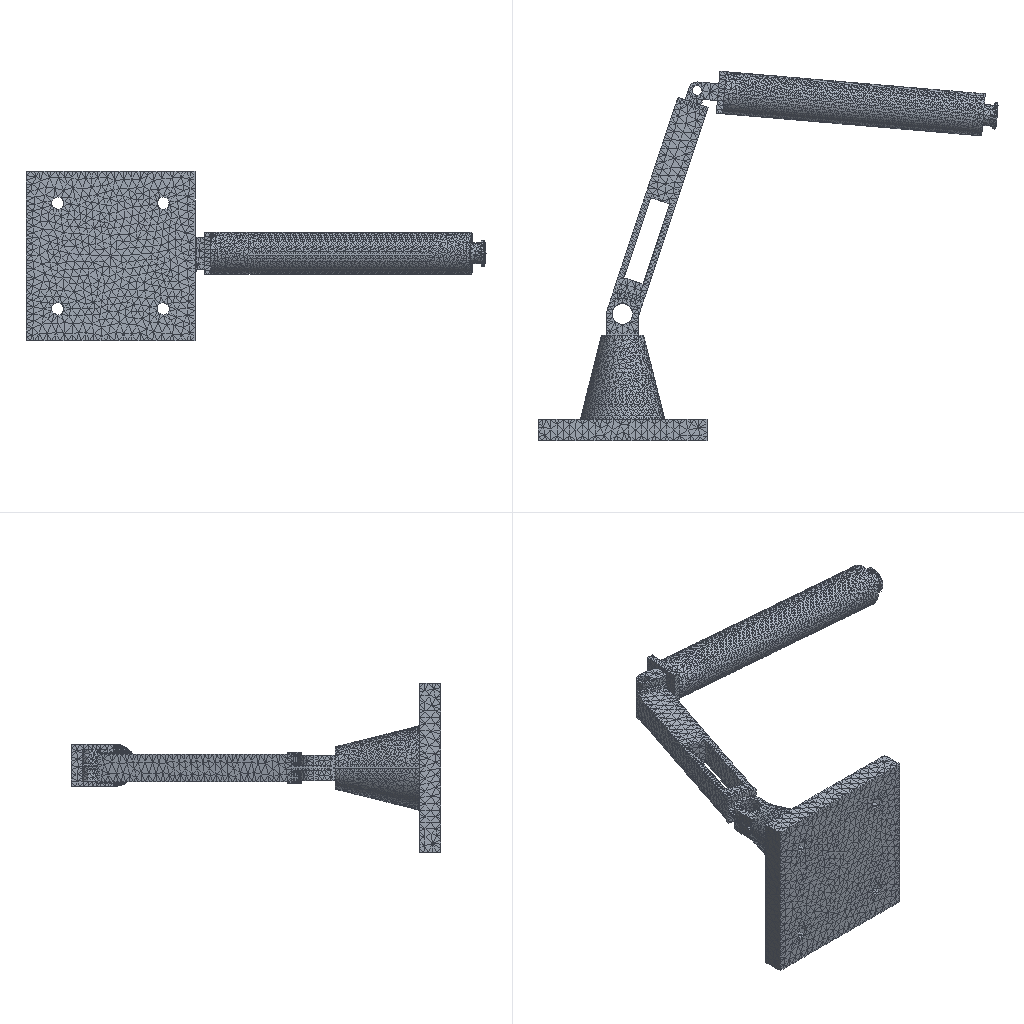Simulation study | ansys workbench
Set-up summary:
category,name,step,type,value,unit,region
solver,ansys_mapdl
solver,version,,,21.1
units,MPA,,stated
analysis,deck,,static,static
load_step,requested,,,1
analysis,nlgeom,,,False
mesh,nodes,,,56505
mesh,elements,,,31911
element_type,ANSYS 187 (type 1),,solid,13480
element_type,ANSYS 187 (type 2),,solid,17937
element_type,ANSYS 174 (type 3),,contact,228
element_type,ANSYS 170 (type 4),,target,228
element_type,ANSYS 154 (type 5),,surface,38
load,load commands in deck,,count,3
bc,support commands in deck,,count,2
named_set,_FIXEDSU,,component
named_set,_FRICSUY,,component
material,1,,in results
material,2,,in results
check,setup vs results,,match,38 surface effect element(s) are not in the reader's mesh and were not compared
Ansys APDL input file, long lists of numbers shortened:
/batch
/config,noeldb,1     ! force off writing results to database
*get,_wallstrt,active,,time,wall
! ANSYS input file written by Workbench version 2021 R1
! File used for geometry attach: D:\仿真\2026.07.04作业分析\模型0706\装配体0706.STEP
/title,____--____ (C5)
! ****** Begin Custom Load Command Snippet ******
/COM, ACT Extensions:
/COM,     LSDYNA, 2021.1
/COM,
! ****** End   Custom Load Command Snippet ******
*DIM,_wb_ProjectScratch_dir,string,248
_wb_ProjectScratch_dir(1) = 'D:\仿真\2026.07.04作业分析\_ProjectScratch\Scr1F88\'
*DIM,_wb_SolverFiles_dir,string,248
_wb_SolverFiles_dir(1) = 'D:\仿真\2026.07.04作业分析\作业分析_files\dp0\SYS-2\MECH\'
*DIM,_wb_userfiles_dir,string,248
_wb_userfiles_dir(1) = 'D:\仿真\2026.07.04作业分析\作业分析_files\user_files\'
/com,--- Data in consistent NMM units. See Solving Units in the help system for more information.
/units,MPA
/nopr
/wb,file,start              !  signify a WB generated input file
/prep7
! Turn off shape checking because checks already performed inside WB mesher.
! See help system for more information.
SHPP,OFF,,NOWARN
/nolist
etcon,set             ! allow ANSYS to choose best KEYOP's for 180x elements, resets any applicable keyopt to MAPDL defaults
/com,*********** Nodes for the whole assembly ***********
nblock,3,,62155
(1i9,3e20.9e3)
        1     2.500000000E+02     6.500000000E+01    -3.005750000E+02
! (56504 more lines like these left out)
-1
/wb,elem,start            !  set before creation of elements
/com,*********** Elements for Body 1 "___0706-FreeParts|NONE" ***********
et,1,187
eblock,19,solid,,13480
(19i9)
        1        1        1        1        0        0        0        0       10        0        1     3000     3829     3017     3722    20851    20955    20841    20850
! (26959 more lines like these left out)
-1
/com,*********** Elements for Body 2 "___0706-FreeParts|NONE[2]" ***********
et,2,187
eblock,19,solid,,17937
(19i9)
        2        2        2        2        0        0        0        0       10        0    13481    25671    29248    25799    28703    38830    39536    38828    38829
! (35873 more lines like these left out)
-1
/wb,elem,end               !  done creating elements
/com,*********** Send User Defined Coordinate System(s) ***********
csys,0
toffst,273.15,  ! Temperature offset from absolute zero
/com,*********** Set Reference Temperature ***********
tref,22.
/wb,mat,start              !  starting to send materials
/com,*********** Send Materials ***********
Temperature = 'TEMP' ! Temperature
MP,DENS,1,7.85e-09,	! tonne mm^-3
MP,ALPX,1,1.2e-05,	! C^-1
MP,C,1,434000000,	! mm^2 s^-2 C^-1
MP,KXX,1,60.5,	! tonne mm s^-3 C^-1
MP,RSVX,1,0.00017,	! ohm mm
MP,EX,1,200000,	! tonne s^-2 mm^-1
MP,NUXY,1,0.3,
MP,MURX,1,10000,
Temperature = 'TEMP' ! Temperature
MP,DENS,2,2.713e-09,	! tonne mm^-3
MP,EX,2,69040,	! tonne s^-2 mm^-1
MP,NUXY,2,0.33,
MP,ALPX,2,2.278e-05,	! C^-1
MP,KXX,2,155.3,	! tonne mm s^-3 C^-1
MP,C,2,915700000,	! mm^2 s^-2 C^-1
/wb,mat,end                !  done sending materials
!************************* Model Summary ********************
!___0706-FreeParts|NONE,	结构钢,	matid,	1
!___0706-FreeParts|NONE[2],	铝合金，锻造，6061，T6,	matid,	2
!************************* End Model Summary ********************
! get the diagonal of the bounding box. Needed later for other things
*get,_xmin,node,,mnloc,x
*get,_ymin,node,,mnloc,y
*get,_zmin,node,,mnloc,z
*get,_xmax,node,,mxloc,x
*get,_ymax,node,,mxloc,y
*get,_zmax,node,,mxloc,z
_ASMDIAG=(_xmax-_xmin)*(_xmax-_xmin)+(_ymax-_ymin)*(_ymax-_ymin)+(_zmax-_zmin)*(_zmax-_zmin)
_ASMDIAG=SQRT(_ASMDIAG)
/wb,contact,start          !  starting to send contact
/com,*********** Create Contact "接触区域" ***********
/com,            Real Constant Set For Above Contact Is 4 & 3
*set,tid,4
*set,cid,3
r,tid
r,cid
et,tid,170
et,cid,174
eblock,10,,,104
(15i9)
    45146        4        4        4        0      156      866      867      867     4869     8828      867     4870
! (103 more lines like these left out)
-1
eblock,10,,,104
(15i9)
    45250        3        3        3        0      156      866      867      867     4869     8828      867     4870
! (103 more lines like these left out)
-1
eblock,10,,,124
(15i9)
    45354        3        4        3        0    24038    24402    24401    24401    29673    31552    24401    29672
! (123 more lines like these left out)
-1
eblock,10,,,124
(15i9)
    45478        4        3        4        0    24038    24402    24401    24401    29673    31552    24401    29672
! (123 more lines like these left out)
-1
keyo,cid,8,2               ! auto create asymmetric contact (from Program Controlled setting)
keyo,cid,10,0              ! adjust contact stiffness each NR iteration (from Program Controlled setting)
keyo,cid,12,5              ! bonded always
keyo,cid,18,1              ! small sliding turned on by application
keyo,cid,2,0               ! augmented Lagrange (from Program Controlled setting)
keyo,cid,4,0               ! on Gauss point (from Program Controlled setting)
keyo,cid,9,1               ! ignore initial gaps/penetration
keyo,cid,7,0               ! No Prediction
rmod,tid,3,10.      ! FKN
rmod,tid,5,0.       ! ICONT
rmod,tid,6,0.       ! PINB
rmod,tid,10,0.      ! CNOF
rmod,tid,12,0.      ! FKT
rmod,tid,36,28      ! WB DSID
rmod,cid,3,10.      ! FKN
rmod,cid,5,0.       ! ICONT
rmod,cid,6,0.       ! PINB
rmod,cid,10,0.      ! CNOF
rmod,cid,12,0.      ! FKT
rmod,cid,36,28      ! WB DSID
nsel,all
esel,all
/wb,contact,end            !  done creating contacts
/golist
/wb,load,start             !  starting to send loads
/com,*********** Fixed Supports ***********
CMBLOCK,_FIXEDSU,NODE,      312
(8i10)
         1         2         3         4         5         6         7         8
! (38 more lines like these left out)
cmsel,s,_FIXEDSU
d,all,all
nsel,all
/com,********* Frictionless Supports Y *********
CMBLOCK,_FRICSUY,NODE,     2389
(8i10)
        21        22        23        24        25        26        59        60
! (298 more lines like these left out)
cmsel,s,_FRICSUY
d,all,uy,0
nsel,all
/com,*********** Define Force Using Surface Effect Elements ***********
local,12,0,0.,0.,0.,0.,0.,0.
csys,0
et,5,154
eblock,10,,,38
(15i9)
    45602        5        5        5       12    24586    27914    25198    25198    32405    36466    25198    32402
! (37 more lines like these left out)
-1
esel,s,type,,5
keyop,5,2,1                ! Apply load in local coordinate system
keyop,5,7,1                ! Use original area so load is constant in large deformation
esel,all
/gst,on,on
fini
*get,_numnode,node,0,count
*get,_numelem,elem,0,count
*get, _MAXELEMNUM, elem, 0, NUM, MAX
*get, _MAXNODENUM, node, 0, NUM, MAX
*get, _MAXELEMTYPE, etyp, 0, NUM, MAX
*get, _MAXREALCONST, real, 0, NUM, MAX
/go
/wb,load,end               !  done creating loads
/com,--- Number of total nodes = %_numnode%
/com,--- Number of contact elements = 494
/com,--- Number of spring elements = 0
/com,--- Number of bearing elements = 0
/com,--- Number of solid elements = 31417
/com,--- Number of condensed parts = 0
/com,--- Number of total elements = %_numelem%
*get,_wallbsol,active,,time,wall
/com,****************************************************************************
/com,*************************    SOLUTION       ********************************
/com,****************************************************************************
/solu
antype,0                   ! static analysis
_thickRatio=  1     ! Ratio of thick parts in the model
eqsl,pcg,1e-8,,,,,,1
cntr,print,1               ! print out contact info and also make no initial contact an error
dmpoption,emat,no             ! Don't combine emat file for DANSYS
dmpoption,esav,no             ! Don't combine esav file for DANSYS
nldiag,cont,iter           ! print out contact info each equilibrium iteration
rescontrol,,none                 ! Do not keep any restart files
/com,****************************************************
/com,******************* SOLVE FOR LS 1 OF 1 ****************
esel,s,type,,5
nsle
sfe,all,1,pres,1,-2.163100572334e-003
sfe,all,2,pres,1,-2.53670115664148e-002
sfe,all,3,pres,1,0.
nsel,all
esel,all
/nopr
/gopr
/nolist
nsub,1,1,1
time,1.
outres,erase
outres,all,none
outres,nsol,all,
outres,rsol,all
outres,eangl,all
outres,etmp,all
outres,veng,all
outres,strs,all,
outres,epel,all,
outres,eppl,all,
outres,cont,all,
! *********** WB SOLVE COMMAND ***********
! check interactive state
*get,ANSINTER_,active,,int
*if,ANSINTER_,ne,0,then
/eof
*endif
solve
/com *************** Write FE CONNECTORS *********
CEWRITE,file,ce,,INTE
/com,****************************************************
/com,*************** FINISHED SOLVE FOR LS 1 *************
*get,_wallasol,active,,time,wall
/nopr
*get,_numnode,node,0,count
*get,_numelem,elem,0,count
*get, _MAXELEMNUM, elem, 0, NUM, MAX
*get, _MAXNODENUM, node, 0, NUM, MAX,,,INTERNAL
*get, _MAXELEMTYPE, etyp, 0, NUM, MAX
*get, _MAXREALCONST, real, 0, NUM, MAX
/gopr
*get,_PCGITER,active,,solu,cgiter
/post1
xmlo,ENCODING,ISO-8859-1
xmlo,parm
/xml,parm,xml
fini
/gopr
*get,_walldone,active,,time,wall
_preptime=(_wallbsol-_wallstrt)*3600
_solvtime=(_wallasol-_wallbsol)*3600
_posttime=(_walldone-_wallasol)*3600
_totaltim=(_walldone-_wallstrt)*3600
*get,_dlbratio,active,0,solu,dlbr
*get,_combtime,active,0,solu,comb
/com,--- Total number of nodes = %_numnode%
/com,--- Total number of elements = %_numelem%
/com,--- Element load balance ratio = %_dlbratio%
/com,--- Time to combine distributed files = %_combtime%
/wb,file,end               ! done with WB generated input
Results summary:
result,analysis,,,static
result,last_loadstep,,,1
result,primary field,,,displacement
result,reaction total,1,FX,12.745,N
result,reaction total,1,FY,149.458,N
result,reaction total,1,FZ,-0.0,N
result,mass,,,0.8826,"NMM: mm, ton, N, s, mV, mA, degC"